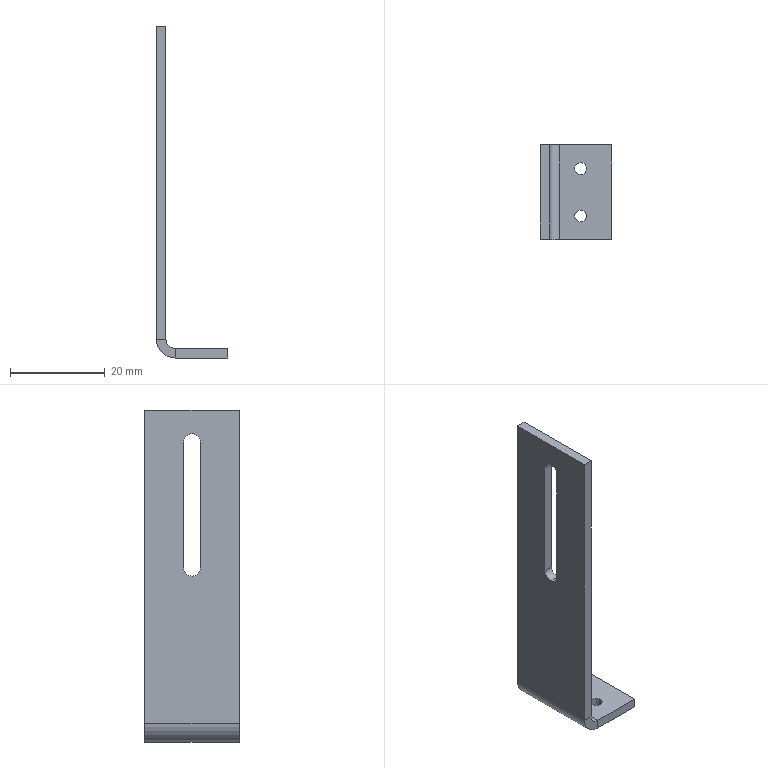Part | STEP file | Slot photoelectric switch bracket 1001 | 1 solid | 23 faces | box 15 x 20 x 70 mm | volume 3044 mm3 | plane 14 | cylinder 9 | commonest cylinder face diameters 2.5 x4 3.5 x3 4 x1 8 x1